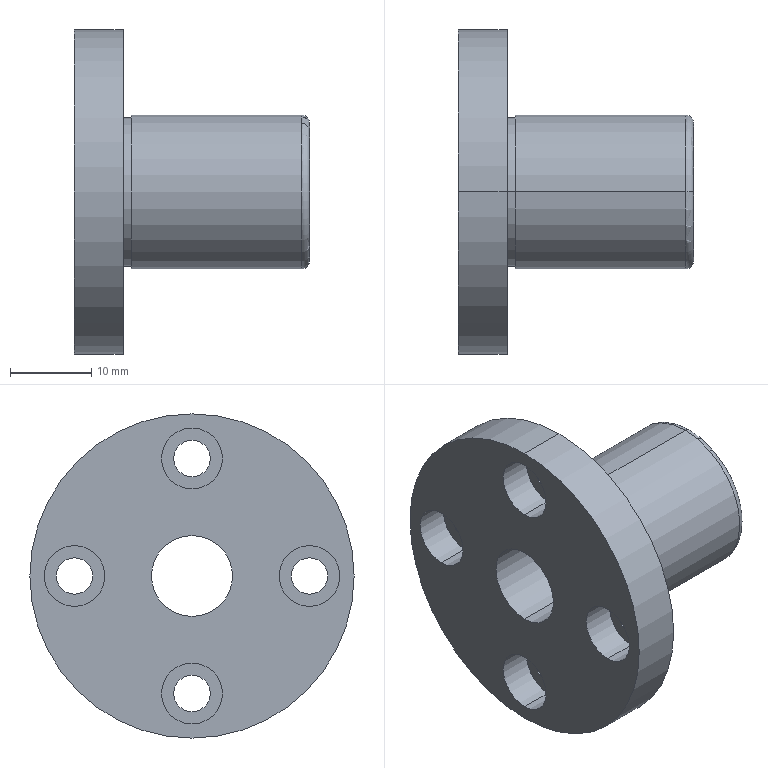Part | SolidWorks | features LPattern 1, RevCut 1, Revolution 1 | 1 solid | 34 faces | box 29 x 40 x 40 mm | volume 10909 mm3 | cylinder 24 | plane 8 | torus 2 | commonest cylinder face diameters 4.5 x8 7.5 x8 10 x2 18.4 x2 19 x2 40 x2
STEP:
#1=CARTESIAN_POINT('',(6.,-14.5,-2.25));
#2=VERTEX_POINT('',#1);
#3=CARTESIAN_POINT('',(6.,-14.5,2.25));
#4=VERTEX_POINT('',#3);
#5=CARTESIAN_POINT('',(6.,-14.5,0.));
#6=DIRECTION('',(-1.,0.,0.));
#7=DIRECTION('',(0.,0.,1.));
#8=AXIS2_PLACEMENT_3D('',#5,#6,#7);
#9=CIRCLE('',#8,2.25);
#10=EDGE_CURVE('',#2,#4,#9,.T.);
#11=ORIENTED_EDGE('',*,*,#10,.F.);
#12=CARTESIAN_POINT('',(4.1,-14.5,-2.25));
#13=VERTEX_POINT('',#12);
#14=CARTESIAN_POINT('',(6.,-14.5,-2.25));
#15=DIRECTION('',(-1.,0.,0.));
#16=VECTOR('',#15,1000.);
#17=LINE('',#14,#16);
#18=EDGE_CURVE('',#2,#13,#17,.T.);
#19=ORIENTED_EDGE('',*,*,#18,.T.);
#20=CARTESIAN_POINT('',(4.1,-14.5,2.25));
#21=VERTEX_POINT('',#20);
#22=CARTESIAN_POINT('',(4.1,-14.5,0.));
#23=DIRECTION('',(-1.,0.,0.));
#24=DIRECTION('',(0.,0.,1.));
#25=AXIS2_PLACEMENT_3D('',#22,#23,#24);
#26=CIRCLE('',#25,2.25);
#27=EDGE_CURVE('',#13,#21,#26,.T.);
#28=ORIENTED_EDGE('',*,*,#27,.T.);
#29=CARTESIAN_POINT('',(6.,-14.5,2.25));
#30=DIRECTION('',(-1.,0.,0.));
#31=VECTOR('',#30,1000.);
#32=LINE('',#29,#31);
#33=EDGE_CURVE('',#4,#21,#32,.T.);
#34=ORIENTED_EDGE('',*,*,#33,.F.);
#35=EDGE_LOOP('',(#11,#19,#28,#34));
#36=FACE_OUTER_BOUND('',#35,.T.);
#37=CARTESIAN_POINT('',(6.,-14.5,0.));
#38=DIRECTION('',(-1.,0.,0.));
#39=DIRECTION('',(0.,0.,1.));
#40=AXIS2_PLACEMENT_3D('',#37,#38,#39);
#41=CYLINDRICAL_SURFACE('',#40,2.25);
#42=ADVANCED_FACE('',(#36),#41,.F.);
#43=CARTESIAN_POINT('',(4.1,-14.5,-3.75));
#44=VERTEX_POINT('',#43);
#45=CARTESIAN_POINT('',(4.1,-14.5,3.75));
#46=VERTEX_POINT('',#45);
#47=CARTESIAN_POINT('',(4.1,-14.5,0.));
#48=DIRECTION('',(-1.,0.,0.));
#49=DIRECTION('',(0.,0.,1.));
#50=AXIS2_PLACEMENT_3D('',#47,#48,#49);
#51=CIRCLE('',#50,3.75);
#52=EDGE_CURVE('',#44,#46,#51,.T.);
#53=ORIENTED_EDGE('',*,*,#52,.F.);
#54=CARTESIAN_POINT('',(0.,-14.5,-3.75));
#55=VERTEX_POINT('',#54);
#56=CARTESIAN_POINT('',(6.,-14.5,-3.75));
#57=DIRECTION('',(-1.,0.,0.));
#58=VECTOR('',#57,1000.);
#59=LINE('',#56,#58);
#60=EDGE_CURVE('',#44,#55,#59,.T.);
#61=ORIENTED_EDGE('',*,*,#60,.T.);
#62=CARTESIAN_POINT('',(0.,-14.5,3.75));
#63=VERTEX_POINT('',#62);
#64=CARTESIAN_POINT('',(0.,-14.5,0.));
#65=DIRECTION('',(-1.,0.,0.));
#66=DIRECTION('',(0.,0.,1.));
#67=AXIS2_PLACEMENT_3D('',#64,#65,#66);
#68=CIRCLE('',#67,3.75);
#69=EDGE_CURVE('',#55,#63,#68,.T.);
#70=ORIENTED_EDGE('',*,*,#69,.T.);
#71=CARTESIAN_POINT('',(6.,-14.5,3.75));
#72=DIRECTION('',(-1.,0.,0.));
#73=VECTOR('',#72,1000.);
#74=LINE('',#71,#73);
#75=EDGE_CURVE('',#46,#63,#74,.T.);
#76=ORIENTED_EDGE('',*,*,#75,.F.);
#77=EDGE_LOOP('',(#53,#61,#70,#76));
#78=FACE_OUTER_BOUND('',#77,.T.);
#79=CARTESIAN_POINT('',(6.,-14.5,0.));
#80=DIRECTION('',(-1.,0.,0.));
#81=DIRECTION('',(0.,0.,1.));
#82=AXIS2_PLACEMENT_3D('',#79,#80,#81);
#83=CYLINDRICAL_SURFACE('',#82,3.75);
#84=ADVANCED_FACE('',(#78),#83,.F.);
#85=CARTESIAN_POINT('',(6.,0.,12.25));
#86=VERTEX_POINT('',#85);
#87=CARTESIAN_POINT('',(6.,0.,16.75));
#88=VERTEX_POINT('',#87);
#89=CARTESIAN_POINT('',(6.,0.,14.5));
#90=DIRECTION('',(-1.,0.,0.));
#91=DIRECTION('',(0.,0.,1.));
#92=AXIS2_PLACEMENT_3D('',#89,#90,#91);
#93=CIRCLE('',#92,2.25);
#94=EDGE_CURVE('',#86,#88,#93,.T.);
#95=ORIENTED_EDGE('',*,*,#94,.F.);
#96=CARTESIAN_POINT('',(4.1,0.,12.25));
#97=VERTEX_POINT('',#96);
#98=CARTESIAN_POINT('',(6.,0.,12.25));
#99=DIRECTION('',(-1.,0.,0.));
#100=VECTOR('',#99,1000.);
#101=LINE('',#98,#100);
#102=EDGE_CURVE('',#86,#97,#101,.T.);
#103=ORIENTED_EDGE('',*,*,#102,.T.);
#104=CARTESIAN_POINT('',(4.1,0.,16.75));
#105=VERTEX_POINT('',#104);
#106=CARTESIAN_POINT('',(4.1,0.,14.5));
#107=DIRECTION('',(-1.,0.,0.));
#108=DIRECTION('',(0.,0.,1.));
#109=AXIS2_PLACEMENT_3D('',#106,#107,#108);
#110=CIRCLE('',#109,2.25);
#111=EDGE_CURVE('',#97,#105,#110,.T.);
#112=ORIENTED_EDGE('',*,*,#111,.T.);
#113=CARTESIAN_POINT('',(6.,0.,16.75));
#114=DIRECTION('',(-1.,0.,0.));
#115=VECTOR('',#114,1000.);
#116=LINE('',#113,#115);
#117=EDGE_CURVE('',#88,#105,#116,.T.);
#118=ORIENTED_EDGE('',*,*,#117,.F.);
#119=EDGE_LOOP('',(#95,#103,#112,#118));
#120=FACE_OUTER_BOUND('',#119,.T.);
#121=CARTESIAN_POINT('',(6.,0.,14.5));
#122=DIRECTION('',(-1.,0.,0.));
#123=DIRECTION('',(0.,0.,1.));
#124=AXIS2_PLACEMENT_3D('',#121,#122,#123);
#125=CYLINDRICAL_SURFACE('',#124,2.25);
#126=ADVANCED_FACE('',(#120),#125,.F.);
#127=CARTESIAN_POINT('',(4.1,0.,10.75));
#128=VERTEX_POINT('',#127);
#129=CARTESIAN_POINT('',(4.1,0.,18.25));
#130=VERTEX_POINT('',#129);
#131=CARTESIAN_POINT('',(4.1,0.,14.5));
#132=DIRECTION('',(-1.,0.,0.));
#133=DIRECTION('',(0.,0.,1.));
#134=AXIS2_PLACEMENT_3D('',#131,#132,#133);
#135=CIRCLE('',#134,3.75);
#136=EDGE_CURVE('',#128,#130,#135,.T.);
#137=ORIENTED_EDGE('',*,*,#136,.F.);
#138=CARTESIAN_POINT('',(0.,0.,10.75));
#139=VERTEX_POINT('',#138);
#140=CARTESIAN_POINT('',(6.,0.,10.75));
#141=DIRECTION('',(-1.,0.,0.));
#142=VECTOR('',#141,1000.);
#143=LINE('',#140,#142);
#144=EDGE_CURVE('',#128,#139,#143,.T.);
#145=ORIENTED_EDGE('',*,*,#144,.T.);
#146=CARTESIAN_POINT('',(0.,0.,18.25));
#147=VERTEX_POINT('',#146);
#148=CARTESIAN_POINT('',(0.,0.,14.5));
#149=DIRECTION('',(-1.,0.,0.));
#150=DIRECTION('',(0.,0.,1.));
#151=AXIS2_PLACEMENT_3D('',#148,#149,#150);
#152=CIRCLE('',#151,3.75);
#153=EDGE_CURVE('',#139,#147,#152,.T.);
#154=ORIENTED_EDGE('',*,*,#153,.T.);
#155=CARTESIAN_POINT('',(6.,0.,18.25));
#156=DIRECTION('',(-1.,0.,0.));
#157=VECTOR('',#156,1000.);
#158=LINE('',#155,#157);
#159=EDGE_CURVE('',#130,#147,#158,.T.);
#160=ORIENTED_EDGE('',*,*,#159,.F.);
#161=EDGE_LOOP('',(#137,#145,#154,#160));
#162=FACE_OUTER_BOUND('',#161,.T.);
#163=CARTESIAN_POINT('',(6.,0.,14.5));
#164=DIRECTION('',(-1.,0.,0.));
#165=DIRECTION('',(0.,0.,1.));
#166=AXIS2_PLACEMENT_3D('',#163,#164,#165);
#167=CYLINDRICAL_SURFACE('',#166,3.75);
#168=ADVANCED_FACE('',(#162),#167,.F.);
#169=CARTESIAN_POINT('',(6.,0.,-16.75));
#170=VERTEX_POINT('',#169);
#171=CARTESIAN_POINT('',(6.,0.,-12.25));
#172=VERTEX_POINT('',#171);
#173=CARTESIAN_POINT('',(6.,0.,-14.5));
#174=DIRECTION('',(-1.,0.,0.));
#175=DIRECTION('',(0.,0.,1.));
#176=AXIS2_PLACEMENT_3D('',#173,#174,#175);
#177=CIRCLE('',#176,2.25);
#178=EDGE_CURVE('',#170,#172,#177,.T.);
#179=ORIENTED_EDGE('',*,*,#178,.F.);
#180=CARTESIAN_POINT('',(4.1,0.,-16.75));
#181=VERTEX_POINT('',#180);
#182=CARTESIAN_POINT('',(6.,0.,-16.75));
#183=DIRECTION('',(-1.,0.,0.));
#184=VECTOR('',#183,1000.);
#185=LINE('',#182,#184);
#186=EDGE_CURVE('',#170,#181,#185,.T.);
#187=ORIENTED_EDGE('',*,*,#186,.T.);
#188=CARTESIAN_POINT('',(4.1,0.,-12.25));
#189=VERTEX_POINT('',#188);
#190=CARTESIAN_POINT('',(4.1,0.,-14.5));
#191=DIRECTION('',(-1.,0.,0.));
#192=DIRECTION('',(0.,0.,1.));
#193=AXIS2_PLACEMENT_3D('',#190,#191,#192);
#194=CIRCLE('',#193,2.25);
#195=EDGE_CURVE('',#181,#189,#194,.T.);
#196=ORIENTED_EDGE('',*,*,#195,.T.);
#197=CARTESIAN_POINT('',(6.,0.,-12.25));
#198=DIRECTION('',(-1.,0.,0.));
#199=VECTOR('',#198,1000.);
#200=LINE('',#197,#199);
#201=EDGE_CURVE('',#172,#189,#200,.T.);
#202=ORIENTED_EDGE('',*,*,#201,.F.);
#203=EDGE_LOOP('',(#179,#187,#196,#202));
#204=FACE_OUTER_BOUND('',#203,.T.);
#205=CARTESIAN_POINT('',(6.,0.,-14.5));
#206=DIRECTION('',(-1.,0.,0.));
#207=DIRECTION('',(0.,0.,1.));
#208=AXIS2_PLACEMENT_3D('',#205,#206,#207);
#209=CYLINDRICAL_SURFACE('',#208,2.25);
#210=ADVANCED_FACE('',(#204),#209,.F.);
#211=CARTESIAN_POINT('',(4.1,0.,-18.25));
#212=VERTEX_POINT('',#211);
#213=CARTESIAN_POINT('',(4.1,0.,-10.75));
#214=VERTEX_POINT('',#213);
#215=CARTESIAN_POINT('',(4.1,0.,-14.5));
#216=DIRECTION('',(-1.,0.,0.));
#217=DIRECTION('',(0.,0.,1.));
#218=AXIS2_PLACEMENT_3D('',#215,#216,#217);
#219=CIRCLE('',#218,3.75);
#220=EDGE_CURVE('',#212,#214,#219,.T.);
#221=ORIENTED_EDGE('',*,*,#220,.F.);
#222=CARTESIAN_POINT('',(0.,0.,-18.25));
#223=VERTEX_POINT('',#222);
#224=CARTESIAN_POINT('',(6.,0.,-18.25));
#225=DIRECTION('',(-1.,0.,0.));
#226=VECTOR('',#225,1000.);
#227=LINE('',#224,#226);
#228=EDGE_CURVE('',#212,#223,#227,.T.);
#229=ORIENTED_EDGE('',*,*,#228,.T.);
#230=CARTESIAN_POINT('',(0.,0.,-10.75));
#231=VERTEX_POINT('',#230);
#232=CARTESIAN_POINT('',(0.,0.,-14.5));
#233=DIRECTION('',(-1.,0.,0.));
#234=DIRECTION('',(0.,0.,1.));
#235=AXIS2_PLACEMENT_3D('',#232,#233,#234);
#236=CIRCLE('',#235,3.75);
#237=EDGE_CURVE('',#223,#231,#236,.T.);
#238=ORIENTED_EDGE('',*,*,#237,.T.);
#239=CARTESIAN_POINT('',(6.,0.,-10.75));
#240=DIRECTION('',(-1.,0.,0.));
#241=VECTOR('',#240,1000.);
#242=LINE('',#239,#241);
#243=EDGE_CURVE('',#214,#231,#242,.T.);
#244=ORIENTED_EDGE('',*,*,#243,.F.);
#245=EDGE_LOOP('',(#221,#229,#238,#244));
#246=FACE_OUTER_BOUND('',#245,.T.);
#247=CARTESIAN_POINT('',(6.,0.,-14.5));
#248=DIRECTION('',(-1.,0.,0.));
#249=DIRECTION('',(0.,0.,1.));
#250=AXIS2_PLACEMENT_3D('',#247,#248,#249);
#251=CYLINDRICAL_SURFACE('',#250,3.75);
#252=ADVANCED_FACE('',(#246),#251,.F.);
#253=CARTESIAN_POINT('',(6.,14.5,-2.25));
#254=VERTEX_POINT('',#253);
#255=CARTESIAN_POINT('',(6.,14.5,2.25));
#256=VERTEX_POINT('',#255);
#257=CARTESIAN_POINT('',(6.,14.5,0.));
#258=DIRECTION('',(-1.,0.,0.));
#259=DIRECTION('',(0.,0.,1.));
#260=AXIS2_PLACEMENT_3D('',#257,#258,#259);
#261=CIRCLE('',#260,2.25);
#262=EDGE_CURVE('',#254,#256,#261,.T.);
#263=ORIENTED_EDGE('',*,*,#262,.F.);
#264=CARTESIAN_POINT('',(4.1,14.5,-2.25));
#265=VERTEX_POINT('',#264);
#266=CARTESIAN_POINT('',(6.,14.5,-2.25));
#267=DIRECTION('',(-1.,0.,0.));
#268=VECTOR('',#267,1000.);
#269=LINE('',#266,#268);
#270=EDGE_CURVE('',#254,#265,#269,.T.);
#271=ORIENTED_EDGE('',*,*,#270,.T.);
#272=CARTESIAN_POINT('',(4.1,14.5,2.25));
#273=VERTEX_POINT('',#272);
#274=CARTESIAN_POINT('',(4.1,14.5,0.));
#275=DIRECTION('',(-1.,0.,0.));
#276=DIRECTION('',(0.,0.,1.));
#277=AXIS2_PLACEMENT_3D('',#274,#275,#276);
#278=CIRCLE('',#277,2.25);
#279=EDGE_CURVE('',#265,#273,#278,.T.);
#280=ORIENTED_EDGE('',*,*,#279,.T.);
#281=CARTESIAN_POINT('',(6.,14.5,2.25));
#282=DIRECTION('',(-1.,0.,0.));
#283=VECTOR('',#282,1000.);
#284=LINE('',#281,#283);
#285=EDGE_CURVE('',#256,#273,#284,.T.);
#286=ORIENTED_EDGE('',*,*,#285,.F.);
#287=EDGE_LOOP('',(#263,#271,#280,#286));
#288=FACE_OUTER_BOUND('',#287,.T.);
#289=CARTESIAN_POINT('',(6.,14.5,0.));
#290=DIRECTION('',(-1.,0.,0.));
#291=DIRECTION('',(0.,0.,1.));
#292=AXIS2_PLACEMENT_3D('',#289,#290,#291);
#293=CYLINDRICAL_SURFACE('',#292,2.25);
#294=ADVANCED_FACE('',(#288),#293,.F.);
#295=CARTESIAN_POINT('',(4.1,14.5,-3.75));
#296=VERTEX_POINT('',#295);
#297=CARTESIAN_POINT('',(4.1,14.5,3.75));
#298=VERTEX_POINT('',#297);
#299=CARTESIAN_POINT('',(4.1,14.5,0.));
#300=DIRECTION('',(-1.,0.,0.));
#301=DIRECTION('',(0.,0.,1.));
#302=AXIS2_PLACEMENT_3D('',#299,#300,#301);
#303=CIRCLE('',#302,3.75);
#304=EDGE_CURVE('',#296,#298,#303,.T.);
#305=ORIENTED_EDGE('',*,*,#304,.F.);
#306=CARTESIAN_POINT('',(0.,14.5,-3.75));
#307=VERTEX_POINT('',#306);
#308=CARTESIAN_POINT('',(6.,14.5,-3.75));
#309=DIRECTION('',(-1.,0.,0.));
#310=VECTOR('',#309,1000.);
#311=LINE('',#308,#310);
#312=EDGE_CURVE('',#296,#307,#311,.T.);
#313=ORIENTED_EDGE('',*,*,#312,.T.);
#314=CARTESIAN_POINT('',(0.,14.5,3.75));
#315=VERTEX_POINT('',#314);
#316=CARTESIAN_POINT('',(0.,14.5,0.));
#317=DIRECTION('',(-1.,0.,0.));
#318=DIRECTION('',(0.,0.,1.));
#319=AXIS2_PLACEMENT_3D('',#316,#317,#318);
#320=CIRCLE('',#319,3.75);
#321=EDGE_CURVE('',#307,#315,#320,.T.);
#322=ORIENTED_EDGE('',*,*,#321,.T.);
#323=CARTESIAN_POINT('',(6.,14.5,3.75));
#324=DIRECTION('',(-1.,0.,0.));
#325=VECTOR('',#324,1000.);
#326=LINE('',#323,#325);
#327=EDGE_CURVE('',#298,#315,#326,.T.);
#328=ORIENTED_EDGE('',*,*,#327,.F.);
#329=EDGE_LOOP('',(#305,#313,#322,#328));
#330=FACE_OUTER_BOUND('',#329,.T.);
#331=CARTESIAN_POINT('',(6.,14.5,0.));
#332=DIRECTION('',(-1.,0.,0.));
#333=DIRECTION('',(0.,0.,1.));
#334=AXIS2_PLACEMENT_3D('',#331,#332,#333);
#335=CYLINDRICAL_SURFACE('',#334,3.75);
#336=ADVANCED_FACE('',(#330),#335,.F.);
#337=CARTESIAN_POINT('',(7.,0.,9.2));
#338=VERTEX_POINT('',#337);
#339=CARTESIAN_POINT('',(7.,0.,-9.2));
#340=VERTEX_POINT('',#339);
#341=CARTESIAN_POINT('',(7.,0.,0.));
#342=DIRECTION('',(-1.,0.,0.));
#343=DIRECTION('',(0.,0.,1.));
#344=AXIS2_PLACEMENT_3D('',#341,#342,#343);
#345=CIRCLE('',#344,9.2);
#346=EDGE_CURVE('',#338,#340,#345,.T.);
#347=ORIENTED_EDGE('',*,*,#346,.T.);
#348=CARTESIAN_POINT('',(6.,0.,-9.2));
#349=VERTEX_POINT('',#348);
#350=CARTESIAN_POINT('',(29.,0.,-9.2));
#351=DIRECTION('',(-1.,0.,0.));
#352=VECTOR('',#351,1000.);
#353=LINE('',#350,#352);
#354=EDGE_CURVE('',#340,#349,#353,.T.);
#355=ORIENTED_EDGE('',*,*,#354,.T.);
#356=CARTESIAN_POINT('',(6.,0.,9.2));
#357=VERTEX_POINT('',#356);
#358=CARTESIAN_POINT('',(6.,0.,0.));
#359=DIRECTION('',(-1.,0.,0.));
#360=DIRECTION('',(0.,0.,1.));
#361=AXIS2_PLACEMENT_3D('',#358,#359,#360);
#362=CIRCLE('',#361,9.2);
#363=EDGE_CURVE('',#357,#349,#362,.T.);
#364=ORIENTED_EDGE('',*,*,#363,.F.);
#365=CARTESIAN_POINT('',(29.,0.,9.2));
#366=DIRECTION('',(-1.,0.,0.));
#367=VECTOR('',#366,1000.);
#368=LINE('',#365,#367);
#369=EDGE_CURVE('',#338,#357,#368,.T.);
#370=ORIENTED_EDGE('',*,*,#369,.F.);
#371=EDGE_LOOP('',(#347,#355,#364,#370));
#372=FACE_OUTER_BOUND('',#371,.T.);
#373=CARTESIAN_POINT('',(29.,0.,0.));
#374=DIRECTION('',(-1.,0.,0.));
#375=DIRECTION('',(0.,0.,1.));
#376=AXIS2_PLACEMENT_3D('',#373,#374,#375);
#377=CYLINDRICAL_SURFACE('',#376,9.2);
#378=ADVANCED_FACE('',(#372),#377,.T.);
#379=CARTESIAN_POINT('',(28.05,0.,9.5));
#380=VERTEX_POINT('',#379);
#381=CARTESIAN_POINT('',(28.05,0.,-9.5));
#382=VERTEX_POINT('',#381);
#383=CARTESIAN_POINT('',(28.05,0.,0.));
#384=DIRECTION('',(-1.,0.,0.));
#385=DIRECTION('',(0.,0.,1.));
#386=AXIS2_PLACEMENT_3D('',#383,#384,#385);
#387=CIRCLE('',#386,9.5);
#388=EDGE_CURVE('',#380,#382,#387,.T.);
#389=ORIENTED_EDGE('',*,*,#388,.T.);
#390=CARTESIAN_POINT('',(7.,0.,-9.5));
#391=VERTEX_POINT('',#390);
#392=CARTESIAN_POINT('',(29.,0.,-9.5));
#393=DIRECTION('',(-1.,0.,0.));
#394=VECTOR('',#393,1000.);
#395=LINE('',#392,#394);
#396=EDGE_CURVE('',#382,#391,#395,.T.);
#397=ORIENTED_EDGE('',*,*,#396,.T.);
#398=CARTESIAN_POINT('',(7.,0.,9.5));
#399=VERTEX_POINT('',#398);
#400=CARTESIAN_POINT('',(7.,0.,0.));
#401=DIRECTION('',(-1.,0.,0.));
#402=DIRECTION('',(0.,0.,1.));
#403=AXIS2_PLACEMENT_3D('',#400,#401,#402);
#404=CIRCLE('',#403,9.5);
#405=EDGE_CURVE('',#399,#391,#404,.T.);
#406=ORIENTED_EDGE('',*,*,#405,.F.);
#407=CARTESIAN_POINT('',(29.,0.,9.5));
#408=DIRECTION('',(-1.,0.,0.));
#409=VECTOR('',#408,1000.);
#410=LINE('',#407,#409);
#411=EDGE_CURVE('',#380,#399,#410,.T.);
#412=ORIENTED_EDGE('',*,*,#411,.F.);
#413=EDGE_LOOP('',(#389,#397,#406,#412));
#414=FACE_OUTER_BOUND('',#413,.T.);
#415=CARTESIAN_POINT('',(29.,0.,0.));
#416=DIRECTION('',(-1.,0.,0.));
#417=DIRECTION('',(0.,0.,1.));
#418=AXIS2_PLACEMENT_3D('',#415,#416,#417);
#419=CYLINDRICAL_SURFACE('',#418,9.5);
#420=ADVANCED_FACE('',(#414),#419,.T.);
#421=CARTESIAN_POINT('',(29.,0.,8.55));
#422=VERTEX_POINT('',#421);
#423=CARTESIAN_POINT('',(29.,0.,-8.55));
#424=VERTEX_POINT('',#423);
#425=CARTESIAN_POINT('',(29.,0.,0.));
#426=DIRECTION('',(-1.,0.,0.));
#427=DIRECTION('',(0.,0.,1.));
#428=AXIS2_PLACEMENT_3D('',#425,#426,#427);
#429=CIRCLE('',#428,8.55);
#430=EDGE_CURVE('',#422,#424,#429,.T.);
#431=ORIENTED_EDGE('',*,*,#430,.T.);
#432=CARTESIAN_POINT('',(28.05,0.,-8.55));
#433=DIRECTION('',(0.,1.,0.));
#434=DIRECTION('',(0.,0.,1.));
#435=AXIS2_PLACEMENT_3D('',#432,#433,#434);
#436=CIRCLE('',#435,0.95);
#437=EDGE_CURVE('',#424,#382,#436,.T.);
#438=ORIENTED_EDGE('',*,*,#437,.T.);
#439=ORIENTED_EDGE('',*,*,#388,.F.);
#440=CARTESIAN_POINT('',(28.05,0.,8.55));
#441=DIRECTION('',(0.,-1.,0.));
#442=DIRECTION('',(0.,0.,-1.));
#443=AXIS2_PLACEMENT_3D('',#440,#441,#442);
#444=CIRCLE('',#443,0.95);
#445=EDGE_CURVE('',#422,#380,#444,.T.);
#446=ORIENTED_EDGE('',*,*,#445,.F.);
#447=EDGE_LOOP('',(#431,#438,#439,#446));
#448=FACE_OUTER_BOUND('',#447,.T.);
#449=CARTESIAN_POINT('',(28.05,0.,0.));
#450=DIRECTION('',(-1.,0.,0.));
#451=DIRECTION('',(0.,0.,1.));
#452=AXIS2_PLACEMENT_3D('',#449,#450,#451);
#453=TOROIDAL_SURFACE('',#452,8.55,0.95);
#454=ADVANCED_FACE('',(#448),#453,.T.);
#455=CARTESIAN_POINT('',(29.,0.,-5.));
#456=VERTEX_POINT('',#455);
#457=CARTESIAN_POINT('',(29.,0.,5.));
#458=VERTEX_POINT('',#457);
#459=CARTESIAN_POINT('',(29.,0.,0.));
#460=DIRECTION('',(-1.,0.,0.));
#461=DIRECTION('',(0.,0.,1.));
#462=AXIS2_PLACEMENT_3D('',#459,#460,#461);
#463=CIRCLE('',#462,5.);
#464=EDGE_CURVE('',#456,#458,#463,.T.);
#465=ORIENTED_EDGE('',*,*,#464,.F.);
#466=CARTESIAN_POINT('',(0.,0.,-5.));
#467=VERTEX_POINT('',#466);
#468=CARTESIAN_POINT('',(29.,0.,-5.));
#469=DIRECTION('',(-1.,0.,0.));
#470=VECTOR('',#469,1000.);
#471=LINE('',#468,#470);
#472=EDGE_CURVE('',#456,#467,#471,.T.);
#473=ORIENTED_EDGE('',*,*,#472,.T.);
#474=CARTESIAN_POINT('',(0.,0.,5.));
#475=VERTEX_POINT('',#474);
#476=CARTESIAN_POINT('',(0.,0.,0.));
#477=DIRECTION('',(-1.,0.,0.));
#478=DIRECTION('',(0.,0.,1.));
#479=AXIS2_PLACEMENT_3D('',#476,#477,#478);
#480=CIRCLE('',#479,5.);
#481=EDGE_CURVE('',#467,#475,#480,.T.);
#482=ORIENTED_EDGE('',*,*,#481,.T.);
#483=CARTESIAN_POINT('',(29.,0.,5.));
#484=DIRECTION('',(-1.,0.,0.));
#485=VECTOR('',#484,1000.);
#486=LINE('',#483,#485);
#487=EDGE_CURVE('',#458,#475,#486,.T.);
#488=ORIENTED_EDGE('',*,*,#487,.F.);
#489=EDGE_LOOP('',(#465,#473,#482,#488));
#490=FACE_OUTER_BOUND('',#489,.T.);
#491=CARTESIAN_POINT('',(29.,0.,0.));
#492=DIRECTION('',(-1.,0.,0.));
#493=DIRECTION('',(0.,0.,1.));
#494=AXIS2_PLACEMENT_3D('',#491,#492,#493);
#495=CYLINDRICAL_SURFACE('',#494,5.);
#496=ADVANCED_FACE('',(#490),#495,.F.);
#497=CARTESIAN_POINT('',(6.,0.,20.));
#498=VERTEX_POINT('',#497);
#499=CARTESIAN_POINT('',(6.,0.,-20.));
#500=VERTEX_POINT('',#499);
#501=CARTESIAN_POINT('',(6.,0.,0.));
#502=DIRECTION('',(-1.,0.,0.));
#503=DIRECTION('',(0.,0.,1.));
#504=AXIS2_PLACEMENT_3D('',#501,#502,#503);
#505=CIRCLE('',#504,20.);
#506=EDGE_CURVE('',#498,#500,#505,.T.);
#507=ORIENTED_EDGE('',*,*,#506,.T.);
#508=CARTESIAN_POINT('',(0.,0.,-20.));
#509=VERTEX_POINT('',#508);
#510=CARTESIAN_POINT('',(29.,0.,-20.));
#511=DIRECTION('',(-1.,0.,0.));
#512=VECTOR('',#511,1000.);
#513=LINE('',#510,#512);
#514=EDGE_CURVE('',#500,#509,#513,.T.);
#515=ORIENTED_EDGE('',*,*,#514,.T.);
#516=CARTESIAN_POINT('',(0.,0.,20.));
#517=VERTEX_POINT('',#516);
#518=CARTESIAN_POINT('',(0.,0.,0.));
#519=DIRECTION('',(-1.,0.,0.));
#520=DIRECTION('',(0.,0.,1.));
#521=AXIS2_PLACEMENT_3D('',#518,#519,#520);
#522=CIRCLE('',#521,20.);
#523=EDGE_CURVE('',#517,#509,#522,.T.);
#524=ORIENTED_EDGE('',*,*,#523,.F.);
#525=CARTESIAN_POINT('',(29.,0.,20.));
#526=DIRECTION('',(-1.,0.,0.));
#527=VECTOR('',#526,1000.);
#528=LINE('',#525,#527);
#529=EDGE_CURVE('',#498,#517,#528,.T.);
#530=ORIENTED_EDGE('',*,*,#529,.F.);
#531=EDGE_LOOP('',(#507,#515,#524,#530));
#532=FACE_OUTER_BOUND('',#531,.T.);
#533=CARTESIAN_POINT('',(29.,0.,0.));
#534=DIRECTION('',(-1.,0.,0.));
#535=DIRECTION('',(0.,0.,1.));
#536=AXIS2_PLACEMENT_3D('',#533,#534,#535);
#537=CYLINDRICAL_SURFACE('',#536,20.);
#538=ADVANCED_FACE('',(#532),#537,.T.);
#539=CARTESIAN_POINT('',(0.,0.,14.5));
#540=DIRECTION('',(-1.,0.,0.));
#541=DIRECTION('',(0.,0.,1.));
#542=AXIS2_PLACEMENT_3D('',#539,#540,#541);
#543=CIRCLE('',#542,3.75);
#544=EDGE_CURVE('',#147,#139,#543,.T.);
#545=ORIENTED_EDGE('',*,*,#544,.F.);
#546=ORIENTED_EDGE('',*,*,#153,.F.);
#547=EDGE_LOOP('',(#545,#546));
#548=FACE_BOUND('',#547,.T.);
#549=CARTESIAN_POINT('',(0.,14.5,0.));
#550=DIRECTION('',(-1.,0.,0.));
#551=DIRECTION('',(0.,0.,1.));
#552=AXIS2_PLACEMENT_3D('',#549,#550,#551);
#553=CIRCLE('',#552,3.75);
#554=EDGE_CURVE('',#315,#307,#553,.T.);
#555=ORIENTED_EDGE('',*,*,#554,.F.);
#556=ORIENTED_EDGE('',*,*,#321,.F.);
#557=EDGE_LOOP('',(#555,#556));
#558=FACE_BOUND('',#557,.T.);
#559=CARTESIAN_POINT('',(0.,0.,0.));
#560=DIRECTION('',(-1.,0.,0.));
#561=DIRECTION('',(0.,0.,1.));
#562=AXIS2_PLACEMENT_3D('',#559,#560,#561);
#563=CIRCLE('',#562,5.);
#564=EDGE_CURVE('',#475,#467,#563,.T.);
#565=ORIENTED_EDGE('',*,*,#564,.F.);
#566=ORIENTED_EDGE('',*,*,#481,.F.);
#567=EDGE_LOOP('',(#565,#566));
#568=FACE_BOUND('',#567,.T.);
#569=ORIENTED_EDGE('',*,*,#523,.T.);
#570=CARTESIAN_POINT('',(0.,0.,0.));
#571=DIRECTION('',(-1.,0.,0.));
#572=DIRECTION('',(0.,0.,1.));
#573=AXIS2_PLACEMENT_3D('',#570,#571,#572);
#574=CIRCLE('',#573,20.);
#575=EDGE_CURVE('',#509,#517,#574,.T.);
#576=ORIENTED_EDGE('',*,*,#575,.T.);
#577=EDGE_LOOP('',(#569,#576));
#578=FACE_OUTER_BOUND('',#577,.T.);
#579=CARTESIAN_POINT('',(0.,0.,-14.5));
#580=DIRECTION('',(-1.,0.,0.));
#581=DIRECTION('',(0.,0.,1.));
#582=AXIS2_PLACEMENT_3D('',#579,#580,#581);
#583=CIRCLE('',#582,3.75);
#584=EDGE_CURVE('',#231,#223,#583,.T.);
#585=ORIENTED_EDGE('',*,*,#584,.F.);
#586=ORIENTED_EDGE('',*,*,#237,.F.);
#587=EDGE_LOOP('',(#585,#586));
#588=FACE_BOUND('',#587,.T.);
#589=CARTESIAN_POINT('',(0.,-14.5,0.));
#590=DIRECTION('',(-1.,0.,0.));
#591=DIRECTION('',(0.,0.,1.));
#592=AXIS2_PLACEMENT_3D('',#589,#590,#591);
#593=CIRCLE('',#592,3.75);
#594=EDGE_CURVE('',#63,#55,#593,.T.);
#595=ORIENTED_EDGE('',*,*,#594,.F.);
#596=ORIENTED_EDGE('',*,*,#69,.F.);
#597=EDGE_LOOP('',(#595,#596));
#598=FACE_BOUND('',#597,.T.);
#599=CARTESIAN_POINT('',(0.,20.,0.));
#600=DIRECTION('',(1.,0.,0.));
#601=DIRECTION('',(0.,0.,-1.));
#602=AXIS2_PLACEMENT_3D('',#599,#600,#601);
#603=PLANE('',#602);
#604=ADVANCED_FACE('',(#548,#558,#568,#578,#588,#598),#603,.F.);
#605=CARTESIAN_POINT('',(6.,0.,14.5));
#606=DIRECTION('',(-1.,0.,0.));
#607=DIRECTION('',(0.,0.,1.));
#608=AXIS2_PLACEMENT_3D('',#605,#606,#607);
#609=CIRCLE('',#608,2.25);
#610=EDGE_CURVE('',#88,#86,#609,.T.);
#611=ORIENTED_EDGE('',*,*,#610,.T.);
#612=ORIENTED_EDGE('',*,*,#94,.T.);
#613=EDGE_LOOP('',(#611,#612));
#614=FACE_BOUND('',#613,.T.);
#615=CARTESIAN_POINT('',(6.,14.5,0.));
#616=DIRECTION('',(-1.,0.,0.));
#617=DIRECTION('',(0.,0.,1.));
#618=AXIS2_PLACEMENT_3D('',#615,#616,#617);
#619=CIRCLE('',#618,2.25);
#620=EDGE_CURVE('',#256,#254,#619,.T.);
#621=ORIENTED_EDGE('',*,*,#620,.T.);
#622=ORIENTED_EDGE('',*,*,#262,.T.);
#623=EDGE_LOOP('',(#621,#622));
#624=FACE_BOUND('',#623,.T.);
#625=ORIENTED_EDGE('',*,*,#506,.F.);
#626=CARTESIAN_POINT('',(6.,0.,0.));
#627=DIRECTION('',(-1.,0.,0.));
#628=DIRECTION('',(0.,0.,1.));
#629=AXIS2_PLACEMENT_3D('',#626,#627,#628);
#630=CIRCLE('',#629,20.);
#631=EDGE_CURVE('',#500,#498,#630,.T.);
#632=ORIENTED_EDGE('',*,*,#631,.F.);
#633=EDGE_LOOP('',(#625,#632));
#634=FACE_OUTER_BOUND('',#633,.T.);
#635=ORIENTED_EDGE('',*,*,#363,.T.);
#636=CARTESIAN_POINT('',(6.,0.,0.));
#637=DIRECTION('',(-1.,0.,0.));
#638=DIRECTION('',(0.,0.,1.));
#639=AXIS2_PLACEMENT_3D('',#636,#637,#638);
#640=CIRCLE('',#639,9.2);
#641=EDGE_CURVE('',#349,#357,#640,.T.);
#642=ORIENTED_EDGE('',*,*,#641,.T.);
#643=EDGE_LOOP('',(#635,#642));
#644=FACE_BOUND('',#643,.T.);
#645=CARTESIAN_POINT('',(6.,0.,-14.5));
#646=DIRECTION('',(-1.,0.,0.));
#647=DIRECTION('',(0.,0.,1.));
#648=AXIS2_PLACEMENT_3D('',#645,#646,#647);
#649=CIRCLE('',#648,2.25);
#650=EDGE_CURVE('',#172,#170,#649,.T.);
#651=ORIENTED_EDGE('',*,*,#650,.T.);
#652=ORIENTED_EDGE('',*,*,#178,.T.);
#653=EDGE_LOOP('',(#651,#652));
#654=FACE_BOUND('',#653,.T.);
#655=CARTESIAN_POINT('',(6.,-14.5,0.));
#656=DIRECTION('',(-1.,0.,0.));
#657=DIRECTION('',(0.,0.,1.));
#658=AXIS2_PLACEMENT_3D('',#655,#656,#657);
#659=CIRCLE('',#658,2.25);
#660=EDGE_CURVE('',#4,#2,#659,.T.);
#661=ORIENTED_EDGE('',*,*,#660,.T.);
#662=ORIENTED_EDGE('',*,*,#10,.T.);
#663=EDGE_LOOP('',(#661,#662));
#664=FACE_BOUND('',#663,.T.);
#665=CARTESIAN_POINT('',(6.,9.2,0.));
#666=DIRECTION('',(-1.,0.,0.));
#667=DIRECTION('',(0.,0.,1.));
#668=AXIS2_PLACEMENT_3D('',#665,#666,#667);
#669=PLANE('',#668);
#670=ADVANCED_FACE('',(#614,#624,#634,#644,#654,#664),#669,.F.);
#671=ORIENTED_EDGE('',*,*,#514,.F.);
#672=ORIENTED_EDGE('',*,*,#631,.T.);
#673=ORIENTED_EDGE('',*,*,#529,.T.);
#674=ORIENTED_EDGE('',*,*,#575,.F.);
#675=EDGE_LOOP('',(#671,#672,#673,#674));
#676=FACE_OUTER_BOUND('',#675,.T.);
#677=CARTESIAN_POINT('',(29.,0.,0.));
#678=DIRECTION('',(-1.,0.,0.));
#679=DIRECTION('',(0.,0.,1.));
#680=AXIS2_PLACEMENT_3D('',#677,#678,#679);
#681=CYLINDRICAL_SURFACE('',#680,20.);
#682=ADVANCED_FACE('',(#676),#681,.T.);
#683=ORIENTED_EDGE('',*,*,#472,.F.);
#684=CARTESIAN_POINT('',(29.,0.,0.));
#685=DIRECTION('',(-1.,0.,0.));
#686=DIRECTION('',(0.,0.,1.));
#687=AXIS2_PLACEMENT_3D('',#684,#685,#686);
#688=CIRCLE('',#687,5.);
#689=EDGE_CURVE('',#458,#456,#688,.T.);
#690=ORIENTED_EDGE('',*,*,#689,.F.);
#691=ORIENTED_EDGE('',*,*,#487,.T.);
#692=ORIENTED_EDGE('',*,*,#564,.T.);
#693=EDGE_LOOP('',(#683,#690,#691,#692));
#694=FACE_OUTER_BOUND('',#693,.T.);
#695=CARTESIAN_POINT('',(29.,0.,0.));
#696=DIRECTION('',(-1.,0.,0.));
#697=DIRECTION('',(0.,0.,1.));
#698=AXIS2_PLACEMENT_3D('',#695,#696,#697);
#699=CYLINDRICAL_SURFACE('',#698,5.);
#700=ADVANCED_FACE('',(#694),#699,.F.);
#701=ORIENTED_EDGE('',*,*,#430,.F.);
#702=CARTESIAN_POINT('',(29.,0.,0.));
#703=DIRECTION('',(-1.,0.,0.));
#704=DIRECTION('',(0.,0.,1.));
#705=AXIS2_PLACEMENT_3D('',#702,#703,#704);
#706=CIRCLE('',#705,8.55);
#707=EDGE_CURVE('',#424,#422,#706,.T.);
#708=ORIENTED_EDGE('',*,*,#707,.F.);
#709=EDGE_LOOP('',(#701,#708));
#710=FACE_OUTER_BOUND('',#709,.T.);
#711=ORIENTED_EDGE('',*,*,#689,.T.);
#712=ORIENTED_EDGE('',*,*,#464,.T.);
#713=EDGE_LOOP('',(#711,#712));
#714=FACE_BOUND('',#713,.T.);
#715=CARTESIAN_POINT('',(29.,5.,0.));
#716=DIRECTION('',(-1.,0.,0.));
#717=DIRECTION('',(0.,0.,1.));
#718=AXIS2_PLACEMENT_3D('',#715,#716,#717);
#719=PLANE('',#718);
#720=ADVANCED_FACE('',(#710,#714),#719,.F.);
#721=ORIENTED_EDGE('',*,*,#437,.F.);
#722=ORIENTED_EDGE('',*,*,#707,.T.);
#723=ORIENTED_EDGE('',*,*,#445,.T.);
#724=CARTESIAN_POINT('',(28.05,0.,0.));
#725=DIRECTION('',(-1.,0.,0.));
#726=DIRECTION('',(0.,0.,1.));
#727=AXIS2_PLACEMENT_3D('',#724,#725,#726);
#728=CIRCLE('',#727,9.5);
#729=EDGE_CURVE('',#382,#380,#728,.T.);
#730=ORIENTED_EDGE('',*,*,#729,.F.);
#731=EDGE_LOOP('',(#721,#722,#723,#730));
#732=FACE_OUTER_BOUND('',#731,.T.);
#733=CARTESIAN_POINT('',(28.05,0.,0.));
#734=DIRECTION('',(-1.,0.,0.));
#735=DIRECTION('',(0.,0.,1.));
#736=AXIS2_PLACEMENT_3D('',#733,#734,#735);
#737=TOROIDAL_SURFACE('',#736,8.55,0.95);
#738=ADVANCED_FACE('',(#732),#737,.T.);
#739=ORIENTED_EDGE('',*,*,#396,.F.);
#740=ORIENTED_EDGE('',*,*,#729,.T.);
#741=ORIENTED_EDGE('',*,*,#411,.T.);
#742=CARTESIAN_POINT('',(7.,0.,0.));
#743=DIRECTION('',(-1.,0.,0.));
#744=DIRECTION('',(0.,0.,1.));
#745=AXIS2_PLACEMENT_3D('',#742,#743,#744);
#746=CIRCLE('',#745,9.5);
#747=EDGE_CURVE('',#391,#399,#746,.T.);
#748=ORIENTED_EDGE('',*,*,#747,.F.);
#749=EDGE_LOOP('',(#739,#740,#741,#748));
#750=FACE_OUTER_BOUND('',#749,.T.);
#751=CARTESIAN_POINT('',(29.,0.,0.));
#752=DIRECTION('',(-1.,0.,0.));
#753=DIRECTION('',(0.,0.,1.));
#754=AXIS2_PLACEMENT_3D('',#751,#752,#753);
#755=CYLINDRICAL_SURFACE('',#754,9.5);
#756=ADVANCED_FACE('',(#750),#755,.T.);
#757=ORIENTED_EDGE('',*,*,#346,.F.);
#758=CARTESIAN_POINT('',(7.,0.,0.));
#759=DIRECTION('',(-1.,0.,0.));
#760=DIRECTION('',(0.,0.,1.));
#761=AXIS2_PLACEMENT_3D('',#758,#759,#760);
#762=CIRCLE('',#761,9.2);
#763=EDGE_CURVE('',#340,#338,#762,.T.);
#764=ORIENTED_EDGE('',*,*,#763,.F.);
#765=EDGE_LOOP('',(#757,#764));
#766=FACE_BOUND('',#765,.T.);
#767=ORIENTED_EDGE('',*,*,#405,.T.);
#768=ORIENTED_EDGE('',*,*,#747,.T.);
#769=EDGE_LOOP('',(#767,#768));
#770=FACE_OUTER_BOUND('',#769,.T.);
#771=CARTESIAN_POINT('',(7.,9.5,0.));
#772=DIRECTION('',(1.,0.,0.));
#773=DIRECTION('',(0.,0.,-1.));
#774=AXIS2_PLACEMENT_3D('',#771,#772,#773);
#775=PLANE('',#774);
#776=ADVANCED_FACE('',(#766,#770),#775,.F.);
#777=ORIENTED_EDGE('',*,*,#354,.F.);
#778=ORIENTED_EDGE('',*,*,#763,.T.);
#779=ORIENTED_EDGE('',*,*,#369,.T.);
#780=ORIENTED_EDGE('',*,*,#641,.F.);
#781=EDGE_LOOP('',(#777,#778,#779,#780));
#782=FACE_OUTER_BOUND('',#781,.T.);
#783=CARTESIAN_POINT('',(29.,0.,0.));
#784=DIRECTION('',(-1.,0.,0.));
#785=DIRECTION('',(0.,0.,1.));
#786=AXIS2_PLACEMENT_3D('',#783,#784,#785);
#787=CYLINDRICAL_SURFACE('',#786,9.2);
#788=ADVANCED_FACE('',(#782),#787,.T.);
#789=ORIENTED_EDGE('',*,*,#312,.F.);
#790=CARTESIAN_POINT('',(4.1,14.5,0.));
#791=DIRECTION('',(-1.,0.,0.));
#792=DIRECTION('',(0.,0.,1.));
#793=AXIS2_PLACEMENT_3D('',#790,#791,#792);
#794=CIRCLE('',#793,3.75);
#795=EDGE_CURVE('',#298,#296,#794,.T.);
#796=ORIENTED_EDGE('',*,*,#795,.F.);
#797=ORIENTED_EDGE('',*,*,#327,.T.);
#798=ORIENTED_EDGE('',*,*,#554,.T.);
#799=EDGE_LOOP('',(#789,#796,#797,#798));
#800=FACE_OUTER_BOUND('',#799,.T.);
#801=CARTESIAN_POINT('',(6.,14.5,0.));
#802=DIRECTION('',(-1.,0.,0.));
#803=DIRECTION('',(0.,0.,1.));
#804=AXIS2_PLACEMENT_3D('',#801,#802,#803);
#805=CYLINDRICAL_SURFACE('',#804,3.75);
#806=ADVANCED_FACE('',(#800),#805,.F.);
#807=ORIENTED_EDGE('',*,*,#795,.T.);
#808=ORIENTED_EDGE('',*,*,#304,.T.);
#809=EDGE_LOOP('',(#807,#808));
#810=FACE_OUTER_BOUND('',#809,.T.);
#811=CARTESIAN_POINT('',(4.1,14.5,0.));
#812=DIRECTION('',(-1.,0.,0.));
#813=DIRECTION('',(0.,0.,1.));
#814=AXIS2_PLACEMENT_3D('',#811,#812,#813);
#815=CIRCLE('',#814,2.25);
#816=EDGE_CURVE('',#273,#265,#815,.T.);
#817=ORIENTED_EDGE('',*,*,#816,.F.);
#818=ORIENTED_EDGE('',*,*,#279,.F.);
#819=EDGE_LOOP('',(#817,#818));
#820=FACE_BOUND('',#819,.T.);
#821=CARTESIAN_POINT('',(4.1,18.25,0.));
#822=DIRECTION('',(-1.,0.,0.));
#823=DIRECTION('',(0.,0.,1.));
#824=AXIS2_PLACEMENT_3D('',#821,#822,#823);
#825=PLANE('',#824);
#826=ADVANCED_FACE('',(#810,#820),#825,.T.);
#827=ORIENTED_EDGE('',*,*,#270,.F.);
#828=ORIENTED_EDGE('',*,*,#620,.F.);
#829=ORIENTED_EDGE('',*,*,#285,.T.);
#830=ORIENTED_EDGE('',*,*,#816,.T.);
#831=EDGE_LOOP('',(#827,#828,#829,#830));
#832=FACE_OUTER_BOUND('',#831,.T.);
#833=CARTESIAN_POINT('',(6.,14.5,0.));
#834=DIRECTION('',(-1.,0.,0.));
#835=DIRECTION('',(0.,0.,1.));
#836=AXIS2_PLACEMENT_3D('',#833,#834,#835);
#837=CYLINDRICAL_SURFACE('',#836,2.25);
#838=ADVANCED_FACE('',(#832),#837,.F.);
#839=ORIENTED_EDGE('',*,*,#228,.F.);
#840=CARTESIAN_POINT('',(4.1,0.,-14.5));
#841=DIRECTION('',(-1.,0.,0.));
#842=DIRECTION('',(0.,0.,1.));
#843=AXIS2_PLACEMENT_3D('',#840,#841,#842);
#844=CIRCLE('',#843,3.75);
#845=EDGE_CURVE('',#214,#212,#844,.T.);
#846=ORIENTED_EDGE('',*,*,#845,.F.);
#847=ORIENTED_EDGE('',*,*,#243,.T.);
#848=ORIENTED_EDGE('',*,*,#584,.T.);
#849=EDGE_LOOP('',(#839,#846,#847,#848));
#850=FACE_OUTER_BOUND('',#849,.T.);
#851=CARTESIAN_POINT('',(6.,0.,-14.5));
#852=DIRECTION('',(-1.,0.,0.));
#853=DIRECTION('',(0.,0.,1.));
#854=AXIS2_PLACEMENT_3D('',#851,#852,#853);
#855=CYLINDRICAL_SURFACE('',#854,3.75);
#856=ADVANCED_FACE('',(#850),#855,.F.);
#857=ORIENTED_EDGE('',*,*,#845,.T.);
#858=ORIENTED_EDGE('',*,*,#220,.T.);
#859=EDGE_LOOP('',(#857,#858));
#860=FACE_OUTER_BOUND('',#859,.T.);
#861=CARTESIAN_POINT('',(4.1,0.,-14.5));
#862=DIRECTION('',(-1.,0.,0.));
#863=DIRECTION('',(0.,0.,1.));
#864=AXIS2_PLACEMENT_3D('',#861,#862,#863);
#865=CIRCLE('',#864,2.25);
#866=EDGE_CURVE('',#189,#181,#865,.T.);
#867=ORIENTED_EDGE('',*,*,#866,.F.);
#868=ORIENTED_EDGE('',*,*,#195,.F.);
#869=EDGE_LOOP('',(#867,#868));
#870=FACE_BOUND('',#869,.T.);
#871=CARTESIAN_POINT('',(4.1,3.75,-14.5));
#872=DIRECTION('',(-1.,0.,0.));
#873=DIRECTION('',(0.,0.,1.));
#874=AXIS2_PLACEMENT_3D('',#871,#872,#873);
#875=PLANE('',#874);
#876=ADVANCED_FACE('',(#860,#870),#875,.T.);
#877=ORIENTED_EDGE('',*,*,#186,.F.);
#878=ORIENTED_EDGE('',*,*,#650,.F.);
#879=ORIENTED_EDGE('',*,*,#201,.T.);
#880=ORIENTED_EDGE('',*,*,#866,.T.);
#881=EDGE_LOOP('',(#877,#878,#879,#880));
#882=FACE_OUTER_BOUND('',#881,.T.);
#883=CARTESIAN_POINT('',(6.,0.,-14.5));
#884=DIRECTION('',(-1.,0.,0.));
#885=DIRECTION('',(0.,0.,1.));
#886=AXIS2_PLACEMENT_3D('',#883,#884,#885);
#887=CYLINDRICAL_SURFACE('',#886,2.25);
#888=ADVANCED_FACE('',(#882),#887,.F.);
#889=ORIENTED_EDGE('',*,*,#144,.F.);
#890=CARTESIAN_POINT('',(4.1,0.,14.5));
#891=DIRECTION('',(-1.,0.,0.));
#892=DIRECTION('',(0.,0.,1.));
#893=AXIS2_PLACEMENT_3D('',#890,#891,#892);
#894=CIRCLE('',#893,3.75);
#895=EDGE_CURVE('',#130,#128,#894,.T.);
#896=ORIENTED_EDGE('',*,*,#895,.F.);
#897=ORIENTED_EDGE('',*,*,#159,.T.);
#898=ORIENTED_EDGE('',*,*,#544,.T.);
#899=EDGE_LOOP('',(#889,#896,#897,#898));
#900=FACE_OUTER_BOUND('',#899,.T.);
#901=CARTESIAN_POINT('',(6.,0.,14.5));
#902=DIRECTION('',(-1.,0.,0.));
#903=DIRECTION('',(0.,0.,1.));
#904=AXIS2_PLACEMENT_3D('',#901,#902,#903);
#905=CYLINDRICAL_SURFACE('',#904,3.75);
#906=ADVANCED_FACE('',(#900),#905,.F.);
#907=ORIENTED_EDGE('',*,*,#895,.T.);
#908=ORIENTED_EDGE('',*,*,#136,.T.);
#909=EDGE_LOOP('',(#907,#908));
#910=FACE_OUTER_BOUND('',#909,.T.);
#911=CARTESIAN_POINT('',(4.1,0.,14.5));
#912=DIRECTION('',(-1.,0.,0.));
#913=DIRECTION('',(0.,0.,1.));
#914=AXIS2_PLACEMENT_3D('',#911,#912,#913);
#915=CIRCLE('',#914,2.25);
#916=EDGE_CURVE('',#105,#97,#915,.T.);
#917=ORIENTED_EDGE('',*,*,#916,.F.);
#918=ORIENTED_EDGE('',*,*,#111,.F.);
#919=EDGE_LOOP('',(#917,#918));
#920=FACE_BOUND('',#919,.T.);
#921=CARTESIAN_POINT('',(4.1,3.75,14.5));
#922=DIRECTION('',(-1.,0.,0.));
#923=DIRECTION('',(0.,0.,1.));
#924=AXIS2_PLACEMENT_3D('',#921,#922,#923);
#925=PLANE('',#924);
#926=ADVANCED_FACE('',(#910,#920),#925,.T.);
#927=ORIENTED_EDGE('',*,*,#102,.F.);
#928=ORIENTED_EDGE('',*,*,#610,.F.);
#929=ORIENTED_EDGE('',*,*,#117,.T.);
#930=ORIENTED_EDGE('',*,*,#916,.T.);
#931=EDGE_LOOP('',(#927,#928,#929,#930));
#932=FACE_OUTER_BOUND('',#931,.T.);
#933=CARTESIAN_POINT('',(6.,0.,14.5));
#934=DIRECTION('',(-1.,0.,0.));
#935=DIRECTION('',(0.,0.,1.));
#936=AXIS2_PLACEMENT_3D('',#933,#934,#935);
#937=CYLINDRICAL_SURFACE('',#936,2.25);
#938=ADVANCED_FACE('',(#932),#937,.F.);
#939=ORIENTED_EDGE('',*,*,#60,.F.);
#940=CARTESIAN_POINT('',(4.1,-14.5,0.));
#941=DIRECTION('',(-1.,0.,0.));
#942=DIRECTION('',(0.,0.,1.));
#943=AXIS2_PLACEMENT_3D('',#940,#941,#942);
#944=CIRCLE('',#943,3.75);
#945=EDGE_CURVE('',#46,#44,#944,.T.);
#946=ORIENTED_EDGE('',*,*,#945,.F.);
#947=ORIENTED_EDGE('',*,*,#75,.T.);
#948=ORIENTED_EDGE('',*,*,#594,.T.);
#949=EDGE_LOOP('',(#939,#946,#947,#948));
#950=FACE_OUTER_BOUND('',#949,.T.);
#951=CARTESIAN_POINT('',(6.,-14.5,0.));
#952=DIRECTION('',(-1.,0.,0.));
#953=DIRECTION('',(0.,0.,1.));
#954=AXIS2_PLACEMENT_3D('',#951,#952,#953);
#955=CYLINDRICAL_SURFACE('',#954,3.75);
#956=ADVANCED_FACE('',(#950),#955,.F.);
#957=ORIENTED_EDGE('',*,*,#945,.T.);
#958=ORIENTED_EDGE('',*,*,#52,.T.);
#959=EDGE_LOOP('',(#957,#958));
#960=FACE_OUTER_BOUND('',#959,.T.);
#961=CARTESIAN_POINT('',(4.1,-14.5,0.));
#962=DIRECTION('',(-1.,0.,0.));
#963=DIRECTION('',(0.,0.,1.));
#964=AXIS2_PLACEMENT_3D('',#961,#962,#963);
#965=CIRCLE('',#964,2.25);
#966=EDGE_CURVE('',#21,#13,#965,.T.);
#967=ORIENTED_EDGE('',*,*,#966,.F.);
#968=ORIENTED_EDGE('',*,*,#27,.F.);
#969=EDGE_LOOP('',(#967,#968));
#970=FACE_BOUND('',#969,.T.);
#971=CARTESIAN_POINT('',(4.1,-10.75,0.));
#972=DIRECTION('',(-1.,0.,0.));
#973=DIRECTION('',(0.,0.,1.));
#974=AXIS2_PLACEMENT_3D('',#971,#972,#973);
#975=PLANE('',#974);
#976=ADVANCED_FACE('',(#960,#970),#975,.T.);
#977=ORIENTED_EDGE('',*,*,#18,.F.);
#978=ORIENTED_EDGE('',*,*,#660,.F.);
#979=ORIENTED_EDGE('',*,*,#33,.T.);
#980=ORIENTED_EDGE('',*,*,#966,.T.);
#981=EDGE_LOOP('',(#977,#978,#979,#980));
#982=FACE_OUTER_BOUND('',#981,.T.);
#983=CARTESIAN_POINT('',(6.,-14.5,0.));
#984=DIRECTION('',(-1.,0.,0.));
#985=DIRECTION('',(0.,0.,1.));
#986=AXIS2_PLACEMENT_3D('',#983,#984,#985);
#987=CYLINDRICAL_SURFACE('',#986,2.25);
#988=ADVANCED_FACE('',(#982),#987,.F.);
#989=CLOSED_SHELL('',(#42,#84,#126,#168,#210,#252,#294,#336,#378,#420,#454,#496,#538,#604,#670,#682,#700,#720,#738,#756,#776,#788,#806,#826,#838,#856,#876,#888,#906,#926,#938,#956,#976,#988));
#990=MANIFOLD_SOLID_BREP('',#989);
#991=CARTESIAN_POINT('',(0.,0.,0.));
#992=DIRECTION('',(0.,0.,1.));
#993=DIRECTION('',(1.,0.,0.));
#994=AXIS2_PLACEMENT_3D('',#991,#992,#993);
#995=(LENGTH_UNIT()NAMED_UNIT(*)SI_UNIT(.MILLI.,.METRE.));
#996=UNCERTAINTY_MEASURE_WITH_UNIT(LENGTH_MEASURE(0.00001),#995,'','');
#997=(NAMED_UNIT(*)PLANE_ANGLE_UNIT()SI_UNIT($,.RADIAN.));
#998=(NAMED_UNIT(*)SI_UNIT($,.STERADIAN.)SOLID_ANGLE_UNIT());
#999=(GEOMETRIC_REPRESENTATION_CONTEXT(3)GLOBAL_UNCERTAINTY_ASSIGNED_CONTEXT((#996))GLOBAL_UNIT_ASSIGNED_CONTEXT((#995,#997,#998))REPRESENTATION_CONTEXT('',''));
#1000=ADVANCED_BREP_SHAPE_REPRESENTATION('',(#990,#994),#999);